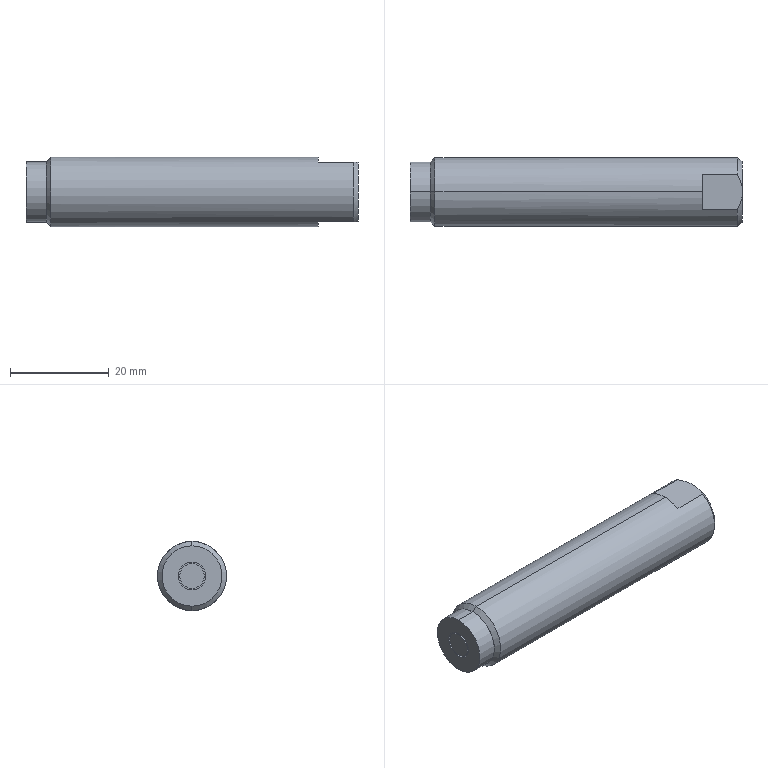Part | SolidWorks | features BaseBody 1 | 1 solid | 21 faces | box 67.1 x 14 x 14 mm | volume 10065 mm3 | plane 9 | cylinder 8 | cone 4 | commonest cylinder face diameters 5 x2 5.6 x2 12.2 x2 14 x2
STEP:
#1=CARTESIAN_POINT('',(59.1,3.606,-6.));
#2=VERTEX_POINT('',#1);
#3=CARTESIAN_POINT('',(59.1,0.,-7.));
#4=VERTEX_POINT('',#3);
#5=CARTESIAN_POINT('',(59.1,0.,0.));
#6=DIRECTION('',(-1.,0.,0.));
#7=DIRECTION('',(0.,0.,1.));
#8=AXIS2_PLACEMENT_3D('',#5,#6,#7);
#9=CIRCLE('',#8,7.);
#10=EDGE_CURVE('',#2,#4,#9,.T.);
#11=ORIENTED_EDGE('',*,*,#10,.T.);
#12=CARTESIAN_POINT('',(5.05,0.,-7.));
#13=VERTEX_POINT('',#12);
#14=CARTESIAN_POINT('',(67.1,0.,-7.));
#15=DIRECTION('',(-1.,0.,0.));
#16=VECTOR('',#15,1000.);
#17=LINE('',#14,#16);
#18=EDGE_CURVE('',#4,#13,#17,.T.);
#19=ORIENTED_EDGE('',*,*,#18,.T.);
#20=CARTESIAN_POINT('',(5.05,0.,7.));
#21=VERTEX_POINT('',#20);
#22=CARTESIAN_POINT('',(5.05,0.,0.));
#23=DIRECTION('',(1.,0.,0.));
#24=DIRECTION('',(0.,0.,1.));
#25=AXIS2_PLACEMENT_3D('',#22,#23,#24);
#26=CIRCLE('',#25,7.);
#27=EDGE_CURVE('',#13,#21,#26,.T.);
#28=ORIENTED_EDGE('',*,*,#27,.T.);
#29=CARTESIAN_POINT('',(59.1,0.,7.));
#30=VERTEX_POINT('',#29);
#31=CARTESIAN_POINT('',(67.1,0.,7.));
#32=DIRECTION('',(-1.,0.,0.));
#33=VECTOR('',#32,1000.);
#34=LINE('',#31,#33);
#35=EDGE_CURVE('',#30,#21,#34,.T.);
#36=ORIENTED_EDGE('',*,*,#35,.F.);
#37=CARTESIAN_POINT('',(59.1,3.606,6.));
#38=VERTEX_POINT('',#37);
#39=CARTESIAN_POINT('',(59.1,0.,0.));
#40=DIRECTION('',(-1.,0.,0.));
#41=DIRECTION('',(0.,0.,1.));
#42=AXIS2_PLACEMENT_3D('',#39,#40,#41);
#43=CIRCLE('',#42,7.);
#44=EDGE_CURVE('',#30,#38,#43,.T.);
#45=ORIENTED_EDGE('',*,*,#44,.T.);
#46=CARTESIAN_POINT('',(66.18,3.606,6.));
#47=VERTEX_POINT('',#46);
#48=CARTESIAN_POINT('',(67.1,3.606,6.));
#49=DIRECTION('',(1.,0.,0.));
#50=VECTOR('',#49,1000.);
#51=LINE('',#48,#50);
#52=EDGE_CURVE('',#38,#47,#51,.T.);
#53=ORIENTED_EDGE('',*,*,#52,.T.);
#54=CARTESIAN_POINT('',(66.18,3.606,-6.));
#55=VERTEX_POINT('',#54);
#56=CARTESIAN_POINT('',(66.18,0.,0.));
#57=DIRECTION('',(-1.,0.,0.));
#58=DIRECTION('',(0.,0.,1.));
#59=AXIS2_PLACEMENT_3D('',#56,#57,#58);
#60=CIRCLE('',#59,7.);
#61=EDGE_CURVE('',#47,#55,#60,.T.);
#62=ORIENTED_EDGE('',*,*,#61,.T.);
#63=CARTESIAN_POINT('',(67.1,3.606,-6.));
#64=DIRECTION('',(-1.,0.,0.));
#65=VECTOR('',#64,1000.);
#66=LINE('',#63,#65);
#67=EDGE_CURVE('',#55,#2,#66,.T.);
#68=ORIENTED_EDGE('',*,*,#67,.T.);
#69=EDGE_LOOP('',(#11,#19,#28,#36,#45,#53,#62,#68));
#70=FACE_OUTER_BOUND('',#69,.T.);
#71=CARTESIAN_POINT('',(67.1,0.,0.));
#72=DIRECTION('',(-1.,0.,0.));
#73=DIRECTION('',(0.,0.,1.));
#74=AXIS2_PLACEMENT_3D('',#71,#72,#73);
#75=CYLINDRICAL_SURFACE('',#74,7.);
#76=ADVANCED_FACE('',(#70),#75,.T.);
#77=CARTESIAN_POINT('',(4.13,0.,-6.08));
#78=VERTEX_POINT('',#77);
#79=CARTESIAN_POINT('',(4.13,0.,6.08));
#80=VERTEX_POINT('',#79);
#81=CARTESIAN_POINT('',(4.13,0.,0.));
#82=DIRECTION('',(1.,0.,0.));
#83=DIRECTION('',(0.,0.,-1.));
#84=AXIS2_PLACEMENT_3D('',#81,#82,#83);
#85=CIRCLE('',#84,6.08);
#86=EDGE_CURVE('',#78,#80,#85,.T.);
#87=ORIENTED_EDGE('',*,*,#86,.T.);
#88=CARTESIAN_POINT('',(5.05,0.,7.));
#89=DIRECTION('',(0.7071,0.,0.7071));
#90=VECTOR('',#89,1000.);
#91=LINE('',#88,#90);
#92=EDGE_CURVE('',#80,#21,#91,.T.);
#93=ORIENTED_EDGE('',*,*,#92,.T.);
#94=ORIENTED_EDGE('',*,*,#27,.F.);
#95=CARTESIAN_POINT('',(5.05,0.,-7.));
#96=DIRECTION('',(0.7071,0.,-0.7071));
#97=VECTOR('',#96,1000.);
#98=LINE('',#95,#97);
#99=EDGE_CURVE('',#78,#13,#98,.T.);
#100=ORIENTED_EDGE('',*,*,#99,.F.);
#101=EDGE_LOOP('',(#87,#93,#94,#100));
#102=FACE_OUTER_BOUND('',#101,.T.);
#103=CARTESIAN_POINT('',(5.05,0.,0.));
#104=DIRECTION('',(1.,0.,0.));
#105=DIRECTION('',(0.,0.,-1.));
#106=AXIS2_PLACEMENT_3D('',#103,#104,#105);
#107=CONICAL_SURFACE('',#106,7.,0.7854);
#108=ADVANCED_FACE('',(#102),#107,.T.);
#109=CARTESIAN_POINT('',(4.13,0.,6.1));
#110=VERTEX_POINT('',#109);
#111=CARTESIAN_POINT('',(4.13,0.,-6.1));
#112=VERTEX_POINT('',#111);
#113=CARTESIAN_POINT('',(4.13,0.,0.));
#114=DIRECTION('',(-1.,0.,0.));
#115=DIRECTION('',(0.,0.,1.));
#116=AXIS2_PLACEMENT_3D('',#113,#114,#115);
#117=CIRCLE('',#116,6.1);
#118=EDGE_CURVE('',#110,#112,#117,.T.);
#119=ORIENTED_EDGE('',*,*,#118,.T.);
#120=CARTESIAN_POINT('',(0.,0.,-6.1));
#121=VERTEX_POINT('',#120);
#122=CARTESIAN_POINT('',(67.1,0.,-6.1));
#123=DIRECTION('',(-1.,0.,0.));
#124=VECTOR('',#123,1000.);
#125=LINE('',#122,#124);
#126=EDGE_CURVE('',#112,#121,#125,.T.);
#127=ORIENTED_EDGE('',*,*,#126,.T.);
#128=CARTESIAN_POINT('',(0.,0.,6.1));
#129=VERTEX_POINT('',#128);
#130=CARTESIAN_POINT('',(0.,0.,0.));
#131=DIRECTION('',(1.,0.,0.));
#132=DIRECTION('',(0.,0.,1.));
#133=AXIS2_PLACEMENT_3D('',#130,#131,#132);
#134=CIRCLE('',#133,6.1);
#135=EDGE_CURVE('',#121,#129,#134,.T.);
#136=ORIENTED_EDGE('',*,*,#135,.T.);
#137=CARTESIAN_POINT('',(67.1,0.,6.1));
#138=DIRECTION('',(-1.,0.,0.));
#139=VECTOR('',#138,1000.);
#140=LINE('',#137,#139);
#141=EDGE_CURVE('',#110,#129,#140,.T.);
#142=ORIENTED_EDGE('',*,*,#141,.F.);
#143=EDGE_LOOP('',(#119,#127,#136,#142));
#144=FACE_OUTER_BOUND('',#143,.T.);
#145=CARTESIAN_POINT('',(67.1,0.,0.));
#146=DIRECTION('',(-1.,0.,0.));
#147=DIRECTION('',(0.,0.,1.));
#148=AXIS2_PLACEMENT_3D('',#145,#146,#147);
#149=CYLINDRICAL_SURFACE('',#148,6.1);
#150=ADVANCED_FACE('',(#144),#149,.T.);
#151=CARTESIAN_POINT('',(0.,0.,-2.8));
#152=VERTEX_POINT('',#151);
#153=CARTESIAN_POINT('',(0.,0.,2.8));
#154=VERTEX_POINT('',#153);
#155=CARTESIAN_POINT('',(0.,0.,0.));
#156=DIRECTION('',(-1.,0.,0.));
#157=DIRECTION('',(0.,0.,-1.));
#158=AXIS2_PLACEMENT_3D('',#155,#156,#157);
#159=CIRCLE('',#158,2.8);
#160=EDGE_CURVE('',#152,#154,#159,.T.);
#161=ORIENTED_EDGE('',*,*,#160,.T.);
#162=CARTESIAN_POINT('',(0.5,0.,2.8));
#163=VERTEX_POINT('',#162);
#164=CARTESIAN_POINT('',(0.5,0.,2.8));
#165=DIRECTION('',(1.,0.,0.));
#166=VECTOR('',#165,1000.);
#167=LINE('',#164,#166);
#168=EDGE_CURVE('',#154,#163,#167,.T.);
#169=ORIENTED_EDGE('',*,*,#168,.T.);
#170=CARTESIAN_POINT('',(0.5,0.,-2.8));
#171=VERTEX_POINT('',#170);
#172=CARTESIAN_POINT('',(0.5,0.,0.));
#173=DIRECTION('',(-1.,0.,0.));
#174=DIRECTION('',(0.,0.,-1.));
#175=AXIS2_PLACEMENT_3D('',#172,#173,#174);
#176=CIRCLE('',#175,2.8);
#177=EDGE_CURVE('',#171,#163,#176,.T.);
#178=ORIENTED_EDGE('',*,*,#177,.F.);
#179=CARTESIAN_POINT('',(0.5,0.,-2.8));
#180=DIRECTION('',(1.,0.,0.));
#181=VECTOR('',#180,1000.);
#182=LINE('',#179,#181);
#183=EDGE_CURVE('',#152,#171,#182,.T.);
#184=ORIENTED_EDGE('',*,*,#183,.F.);
#185=EDGE_LOOP('',(#161,#169,#178,#184));
#186=FACE_OUTER_BOUND('',#185,.T.);
#187=CARTESIAN_POINT('',(0.5,0.,0.));
#188=DIRECTION('',(1.,0.,0.));
#189=DIRECTION('',(0.,0.,-1.));
#190=AXIS2_PLACEMENT_3D('',#187,#188,#189);
#191=CYLINDRICAL_SURFACE('',#190,2.8);
#192=ADVANCED_FACE('',(#186),#191,.F.);
#193=CARTESIAN_POINT('',(0.,0.,-2.5));
#194=VERTEX_POINT('',#193);
#195=CARTESIAN_POINT('',(0.,0.,2.5));
#196=VERTEX_POINT('',#195);
#197=CARTESIAN_POINT('',(0.,0.,0.));
#198=DIRECTION('',(1.,0.,0.));
#199=DIRECTION('',(0.,0.,-1.));
#200=AXIS2_PLACEMENT_3D('',#197,#198,#199);
#201=CIRCLE('',#200,2.5);
#202=EDGE_CURVE('',#194,#196,#201,.T.);
#203=ORIENTED_EDGE('',*,*,#202,.T.);
#204=CARTESIAN_POINT('',(0.5,0.,2.5));
#205=VERTEX_POINT('',#204);
#206=CARTESIAN_POINT('',(0.5,0.,2.5));
#207=DIRECTION('',(1.,0.,0.));
#208=VECTOR('',#207,1000.);
#209=LINE('',#206,#208);
#210=EDGE_CURVE('',#196,#205,#209,.T.);
#211=ORIENTED_EDGE('',*,*,#210,.T.);
#212=CARTESIAN_POINT('',(0.5,0.,-2.5));
#213=VERTEX_POINT('',#212);
#214=CARTESIAN_POINT('',(0.5,0.,0.));
#215=DIRECTION('',(-1.,0.,0.));
#216=DIRECTION('',(0.,0.,-1.));
#217=AXIS2_PLACEMENT_3D('',#214,#215,#216);
#218=CIRCLE('',#217,2.5);
#219=EDGE_CURVE('',#205,#213,#218,.T.);
#220=ORIENTED_EDGE('',*,*,#219,.T.);
#221=CARTESIAN_POINT('',(0.5,0.,-2.5));
#222=DIRECTION('',(1.,0.,0.));
#223=VECTOR('',#222,1000.);
#224=LINE('',#221,#223);
#225=EDGE_CURVE('',#194,#213,#224,.T.);
#226=ORIENTED_EDGE('',*,*,#225,.F.);
#227=EDGE_LOOP('',(#203,#211,#220,#226));
#228=FACE_OUTER_BOUND('',#227,.T.);
#229=CARTESIAN_POINT('',(0.5,0.,0.));
#230=DIRECTION('',(1.,0.,0.));
#231=DIRECTION('',(0.,0.,-1.));
#232=AXIS2_PLACEMENT_3D('',#229,#230,#231);
#233=CYLINDRICAL_SURFACE('',#232,2.5);
#234=ADVANCED_FACE('',(#228),#233,.T.);
#235=ORIENTED_EDGE('',*,*,#18,.F.);
#236=CARTESIAN_POINT('',(59.1,-3.606,-6.));
#237=VERTEX_POINT('',#236);
#238=CARTESIAN_POINT('',(59.1,0.,0.));
#239=DIRECTION('',(-1.,0.,0.));
#240=DIRECTION('',(0.,0.,1.));
#241=AXIS2_PLACEMENT_3D('',#238,#239,#240);
#242=CIRCLE('',#241,7.);
#243=EDGE_CURVE('',#4,#237,#242,.T.);
#244=ORIENTED_EDGE('',*,*,#243,.T.);
#245=CARTESIAN_POINT('',(66.18,-3.606,-6.));
#246=VERTEX_POINT('',#245);
#247=CARTESIAN_POINT('',(67.1,-3.606,-6.));
#248=DIRECTION('',(1.,0.,0.));
#249=VECTOR('',#248,1000.);
#250=LINE('',#247,#249);
#251=EDGE_CURVE('',#237,#246,#250,.T.);
#252=ORIENTED_EDGE('',*,*,#251,.T.);
#253=CARTESIAN_POINT('',(66.18,-3.606,6.));
#254=VERTEX_POINT('',#253);
#255=CARTESIAN_POINT('',(66.18,0.,0.));
#256=DIRECTION('',(-1.,0.,0.));
#257=DIRECTION('',(0.,0.,1.));
#258=AXIS2_PLACEMENT_3D('',#255,#256,#257);
#259=CIRCLE('',#258,7.);
#260=EDGE_CURVE('',#246,#254,#259,.T.);
#261=ORIENTED_EDGE('',*,*,#260,.T.);
#262=CARTESIAN_POINT('',(59.1,-3.606,6.));
#263=VERTEX_POINT('',#262);
#264=CARTESIAN_POINT('',(67.1,-3.606,6.));
#265=DIRECTION('',(-1.,0.,0.));
#266=VECTOR('',#265,1000.);
#267=LINE('',#264,#266);
#268=EDGE_CURVE('',#254,#263,#267,.T.);
#269=ORIENTED_EDGE('',*,*,#268,.T.);
#270=CARTESIAN_POINT('',(59.1,0.,0.));
#271=DIRECTION('',(-1.,0.,0.));
#272=DIRECTION('',(0.,0.,1.));
#273=AXIS2_PLACEMENT_3D('',#270,#271,#272);
#274=CIRCLE('',#273,7.);
#275=EDGE_CURVE('',#263,#30,#274,.T.);
#276=ORIENTED_EDGE('',*,*,#275,.T.);
#277=ORIENTED_EDGE('',*,*,#35,.T.);
#278=CARTESIAN_POINT('',(5.05,0.,0.));
#279=DIRECTION('',(1.,0.,0.));
#280=DIRECTION('',(0.,0.,1.));
#281=AXIS2_PLACEMENT_3D('',#278,#279,#280);
#282=CIRCLE('',#281,7.);
#283=EDGE_CURVE('',#21,#13,#282,.T.);
#284=ORIENTED_EDGE('',*,*,#283,.T.);
#285=EDGE_LOOP('',(#235,#244,#252,#261,#269,#276,#277,#284));
#286=FACE_OUTER_BOUND('',#285,.T.);
#287=CARTESIAN_POINT('',(67.1,0.,0.));
#288=DIRECTION('',(-1.,0.,0.));
#289=DIRECTION('',(0.,0.,1.));
#290=AXIS2_PLACEMENT_3D('',#287,#288,#289);
#291=CYLINDRICAL_SURFACE('',#290,7.);
#292=ADVANCED_FACE('',(#286),#291,.T.);
#293=ORIENTED_EDGE('',*,*,#92,.F.);
#294=CARTESIAN_POINT('',(4.13,0.,0.));
#295=DIRECTION('',(1.,0.,0.));
#296=DIRECTION('',(0.,0.,-1.));
#297=AXIS2_PLACEMENT_3D('',#294,#295,#296);
#298=CIRCLE('',#297,6.08);
#299=EDGE_CURVE('',#80,#78,#298,.T.);
#300=ORIENTED_EDGE('',*,*,#299,.T.);
#301=ORIENTED_EDGE('',*,*,#99,.T.);
#302=ORIENTED_EDGE('',*,*,#283,.F.);
#303=EDGE_LOOP('',(#293,#300,#301,#302));
#304=FACE_OUTER_BOUND('',#303,.T.);
#305=CARTESIAN_POINT('',(5.05,0.,0.));
#306=DIRECTION('',(1.,0.,0.));
#307=DIRECTION('',(0.,0.,-1.));
#308=AXIS2_PLACEMENT_3D('',#305,#306,#307);
#309=CONICAL_SURFACE('',#308,7.,0.7854);
#310=ADVANCED_FACE('',(#304),#309,.T.);
#311=CARTESIAN_POINT('',(59.1,3.606,6.));
#312=DIRECTION('',(0.,-1.,0.));
#313=VECTOR('',#312,1000.);
#314=LINE('',#311,#313);
#315=EDGE_CURVE('',#38,#263,#314,.T.);
#316=ORIENTED_EDGE('',*,*,#315,.T.);
#317=ORIENTED_EDGE('',*,*,#268,.F.);
#318=CARTESIAN_POINT('',(67.1,-0.9831,6.));
#319=VERTEX_POINT('',#318);
#320=CARTESIAN_POINT('',(66.18,-3.606,6.));
#321=CARTESIAN_POINT('',(66.394,-3.19,6.));
#322=CARTESIAN_POINT('',(66.586,-2.766,6.));
#323=CARTESIAN_POINT('',(66.901,-1.895,6.));
#324=CARTESIAN_POINT('',(67.025,-1.448,6.));
#325=CARTESIAN_POINT('',(67.1,-0.9831,6.));
#326=B_SPLINE_CURVE_WITH_KNOTS('',3,(#320,#321,#322,#323,#324,#325),.UNSPECIFIED.,.F.,.F.,(4,2,4),(0.,0.00139,0.002779),.UNSPECIFIED.);
#327=EDGE_CURVE('',#254,#319,#326,.T.);
#328=ORIENTED_EDGE('',*,*,#327,.T.);
#329=CARTESIAN_POINT('',(67.1,0.9831,6.));
#330=VERTEX_POINT('',#329);
#331=CARTESIAN_POINT('',(67.1,3.606,6.));
#332=DIRECTION('',(0.,1.,0.));
#333=VECTOR('',#332,1000.);
#334=LINE('',#331,#333);
#335=EDGE_CURVE('',#319,#330,#334,.T.);
#336=ORIENTED_EDGE('',*,*,#335,.T.);
#337=CARTESIAN_POINT('',(67.1,0.9831,6.));
#338=CARTESIAN_POINT('',(67.025,1.448,6.));
#339=CARTESIAN_POINT('',(66.901,1.895,6.));
#340=CARTESIAN_POINT('',(66.586,2.766,6.));
#341=CARTESIAN_POINT('',(66.394,3.19,6.));
#342=CARTESIAN_POINT('',(66.18,3.606,6.));
#343=B_SPLINE_CURVE_WITH_KNOTS('',3,(#337,#338,#339,#340,#341,#342),.UNSPECIFIED.,.F.,.F.,(4,2,4),(0.,0.00139,0.002779),.UNSPECIFIED.);
#344=EDGE_CURVE('',#330,#47,#343,.T.);
#345=ORIENTED_EDGE('',*,*,#344,.T.);
#346=ORIENTED_EDGE('',*,*,#52,.F.);
#347=EDGE_LOOP('',(#316,#317,#328,#336,#345,#346));
#348=FACE_OUTER_BOUND('',#347,.T.);
#349=CARTESIAN_POINT('',(59.1,3.606,6.));
#350=DIRECTION('',(0.,0.,1.));
#351=DIRECTION('',(1.,0.,0.));
#352=AXIS2_PLACEMENT_3D('',#349,#350,#351);
#353=PLANE('',#352);
#354=ADVANCED_FACE('',(#348),#353,.T.);
#355=ORIENTED_EDGE('',*,*,#275,.F.);
#356=ORIENTED_EDGE('',*,*,#315,.F.);
#357=ORIENTED_EDGE('',*,*,#44,.F.);
#358=EDGE_LOOP('',(#355,#356,#357));
#359=FACE_OUTER_BOUND('',#358,.T.);
#360=CARTESIAN_POINT('',(59.1,0.,0.));
#361=DIRECTION('',(1.,0.,0.));
#362=DIRECTION('',(0.,0.,-1.));
#363=AXIS2_PLACEMENT_3D('',#360,#361,#362);
#364=PLANE('',#363);
#365=ADVANCED_FACE('',(#359),#364,.T.);
#366=ORIENTED_EDGE('',*,*,#327,.F.);
#367=ORIENTED_EDGE('',*,*,#260,.F.);
#368=CARTESIAN_POINT('',(67.1,-0.9831,-6.));
#369=VERTEX_POINT('',#368);
#370=CARTESIAN_POINT('',(66.18,-3.606,-6.));
#371=CARTESIAN_POINT('',(66.394,-3.19,-6.));
#372=CARTESIAN_POINT('',(66.586,-2.766,-6.));
#373=CARTESIAN_POINT('',(66.901,-1.895,-6.));
#374=CARTESIAN_POINT('',(67.025,-1.448,-6.));
#375=CARTESIAN_POINT('',(67.1,-0.9831,-6.));
#376=B_SPLINE_CURVE_WITH_KNOTS('',3,(#370,#371,#372,#373,#374,#375),.UNSPECIFIED.,.F.,.F.,(4,2,4),(0.,0.00139,0.002779),.UNSPECIFIED.);
#377=EDGE_CURVE('',#246,#369,#376,.T.);
#378=ORIENTED_EDGE('',*,*,#377,.T.);
#379=CARTESIAN_POINT('',(67.1,0.,0.));
#380=DIRECTION('',(-1.,0.,0.));
#381=DIRECTION('',(0.,0.,1.));
#382=AXIS2_PLACEMENT_3D('',#379,#380,#381);
#383=CIRCLE('',#382,6.08);
#384=EDGE_CURVE('',#369,#319,#383,.T.);
#385=ORIENTED_EDGE('',*,*,#384,.T.);
#386=EDGE_LOOP('',(#366,#367,#378,#385));
#387=FACE_OUTER_BOUND('',#386,.T.);
#388=CARTESIAN_POINT('',(66.18,0.,0.));
#389=DIRECTION('',(-1.,0.,0.));
#390=DIRECTION('',(0.,0.,1.));
#391=AXIS2_PLACEMENT_3D('',#388,#389,#390);
#392=CONICAL_SURFACE('',#391,7.,0.7854);
#393=ADVANCED_FACE('',(#387),#392,.T.);
#394=CARTESIAN_POINT('',(59.1,-3.606,-6.));
#395=DIRECTION('',(0.,1.,0.));
#396=VECTOR('',#395,1000.);
#397=LINE('',#394,#396);
#398=EDGE_CURVE('',#237,#2,#397,.T.);
#399=ORIENTED_EDGE('',*,*,#398,.T.);
#400=ORIENTED_EDGE('',*,*,#67,.F.);
#401=CARTESIAN_POINT('',(67.1,0.9831,-6.));
#402=VERTEX_POINT('',#401);
#403=CARTESIAN_POINT('',(66.18,3.606,-6.));
#404=CARTESIAN_POINT('',(66.394,3.19,-6.));
#405=CARTESIAN_POINT('',(66.586,2.766,-6.));
#406=CARTESIAN_POINT('',(66.901,1.895,-6.));
#407=CARTESIAN_POINT('',(67.025,1.448,-6.));
#408=CARTESIAN_POINT('',(67.1,0.9831,-6.));
#409=B_SPLINE_CURVE_WITH_KNOTS('',3,(#403,#404,#405,#406,#407,#408),.UNSPECIFIED.,.F.,.F.,(4,2,4),(0.,0.00139,0.002779),.UNSPECIFIED.);
#410=EDGE_CURVE('',#55,#402,#409,.T.);
#411=ORIENTED_EDGE('',*,*,#410,.T.);
#412=CARTESIAN_POINT('',(67.1,-3.606,-6.));
#413=DIRECTION('',(0.,-1.,0.));
#414=VECTOR('',#413,1000.);
#415=LINE('',#412,#414);
#416=EDGE_CURVE('',#402,#369,#415,.T.);
#417=ORIENTED_EDGE('',*,*,#416,.T.);
#418=ORIENTED_EDGE('',*,*,#377,.F.);
#419=ORIENTED_EDGE('',*,*,#251,.F.);
#420=EDGE_LOOP('',(#399,#400,#411,#417,#418,#419));
#421=FACE_OUTER_BOUND('',#420,.T.);
#422=CARTESIAN_POINT('',(59.1,-3.606,-6.));
#423=DIRECTION('',(0.,0.,-1.));
#424=DIRECTION('',(-1.,0.,0.));
#425=AXIS2_PLACEMENT_3D('',#422,#423,#424);
#426=PLANE('',#425);
#427=ADVANCED_FACE('',(#421),#426,.T.);
#428=ORIENTED_EDGE('',*,*,#10,.F.);
#429=ORIENTED_EDGE('',*,*,#398,.F.);
#430=ORIENTED_EDGE('',*,*,#243,.F.);
#431=EDGE_LOOP('',(#428,#429,#430));
#432=FACE_OUTER_BOUND('',#431,.T.);
#433=CARTESIAN_POINT('',(59.1,0.,0.));
#434=DIRECTION('',(1.,0.,0.));
#435=DIRECTION('',(0.,0.,-1.));
#436=AXIS2_PLACEMENT_3D('',#433,#434,#435);
#437=PLANE('',#436);
#438=ADVANCED_FACE('',(#432),#437,.T.);
#439=ORIENTED_EDGE('',*,*,#410,.F.);
#440=ORIENTED_EDGE('',*,*,#61,.F.);
#441=ORIENTED_EDGE('',*,*,#344,.F.);
#442=CARTESIAN_POINT('',(67.1,0.,0.));
#443=DIRECTION('',(-1.,0.,0.));
#444=DIRECTION('',(0.,0.,1.));
#445=AXIS2_PLACEMENT_3D('',#442,#443,#444);
#446=CIRCLE('',#445,6.08);
#447=EDGE_CURVE('',#330,#402,#446,.T.);
#448=ORIENTED_EDGE('',*,*,#447,.T.);
#449=EDGE_LOOP('',(#439,#440,#441,#448));
#450=FACE_OUTER_BOUND('',#449,.T.);
#451=CARTESIAN_POINT('',(66.18,0.,0.));
#452=DIRECTION('',(-1.,0.,0.));
#453=DIRECTION('',(0.,0.,1.));
#454=AXIS2_PLACEMENT_3D('',#451,#452,#453);
#455=CONICAL_SURFACE('',#454,7.,0.7854);
#456=ADVANCED_FACE('',(#450),#455,.T.);
#457=ORIENTED_EDGE('',*,*,#118,.F.);
#458=CARTESIAN_POINT('',(4.13,0.,0.));
#459=DIRECTION('',(-1.,0.,0.));
#460=DIRECTION('',(0.,0.,1.));
#461=AXIS2_PLACEMENT_3D('',#458,#459,#460);
#462=CIRCLE('',#461,6.1);
#463=EDGE_CURVE('',#112,#110,#462,.T.);
#464=ORIENTED_EDGE('',*,*,#463,.F.);
#465=EDGE_LOOP('',(#457,#464));
#466=FACE_OUTER_BOUND('',#465,.T.);
#467=ORIENTED_EDGE('',*,*,#86,.F.);
#468=ORIENTED_EDGE('',*,*,#299,.F.);
#469=EDGE_LOOP('',(#467,#468));
#470=FACE_BOUND('',#469,.T.);
#471=CARTESIAN_POINT('',(4.13,6.1,0.));
#472=DIRECTION('',(-1.,0.,0.));
#473=DIRECTION('',(0.,0.,1.));
#474=AXIS2_PLACEMENT_3D('',#471,#472,#473);
#475=PLANE('',#474);
#476=ADVANCED_FACE('',(#466,#470),#475,.F.);
#477=ORIENTED_EDGE('',*,*,#447,.F.);
#478=ORIENTED_EDGE('',*,*,#335,.F.);
#479=ORIENTED_EDGE('',*,*,#384,.F.);
#480=ORIENTED_EDGE('',*,*,#416,.F.);
#481=EDGE_LOOP('',(#477,#478,#479,#480));
#482=FACE_OUTER_BOUND('',#481,.T.);
#483=CARTESIAN_POINT('',(67.1,6.08,0.));
#484=DIRECTION('',(-1.,0.,0.));
#485=DIRECTION('',(0.,0.,1.));
#486=AXIS2_PLACEMENT_3D('',#483,#484,#485);
#487=PLANE('',#486);
#488=ADVANCED_FACE('',(#482),#487,.F.);
#489=ORIENTED_EDGE('',*,*,#126,.F.);
#490=ORIENTED_EDGE('',*,*,#463,.T.);
#491=ORIENTED_EDGE('',*,*,#141,.T.);
#492=CARTESIAN_POINT('',(0.,0.,0.));
#493=DIRECTION('',(1.,0.,0.));
#494=DIRECTION('',(0.,0.,1.));
#495=AXIS2_PLACEMENT_3D('',#492,#493,#494);
#496=CIRCLE('',#495,6.1);
#497=EDGE_CURVE('',#129,#121,#496,.T.);
#498=ORIENTED_EDGE('',*,*,#497,.T.);
#499=EDGE_LOOP('',(#489,#490,#491,#498));
#500=FACE_OUTER_BOUND('',#499,.T.);
#501=CARTESIAN_POINT('',(67.1,0.,0.));
#502=DIRECTION('',(-1.,0.,0.));
#503=DIRECTION('',(0.,0.,1.));
#504=AXIS2_PLACEMENT_3D('',#501,#502,#503);
#505=CYLINDRICAL_SURFACE('',#504,6.1);
#506=ADVANCED_FACE('',(#500),#505,.T.);
#507=ORIENTED_EDGE('',*,*,#160,.F.);
#508=CARTESIAN_POINT('',(0.,0.,0.));
#509=DIRECTION('',(-1.,0.,0.));
#510=DIRECTION('',(0.,0.,-1.));
#511=AXIS2_PLACEMENT_3D('',#508,#509,#510);
#512=CIRCLE('',#511,2.8);
#513=EDGE_CURVE('',#154,#152,#512,.T.);
#514=ORIENTED_EDGE('',*,*,#513,.F.);
#515=EDGE_LOOP('',(#507,#514));
#516=FACE_BOUND('',#515,.T.);
#517=ORIENTED_EDGE('',*,*,#497,.F.);
#518=ORIENTED_EDGE('',*,*,#135,.F.);
#519=EDGE_LOOP('',(#517,#518));
#520=FACE_OUTER_BOUND('',#519,.T.);
#521=CARTESIAN_POINT('',(0.,0.,0.));
#522=DIRECTION('',(1.,0.,0.));
#523=DIRECTION('',(0.,0.,-1.));
#524=AXIS2_PLACEMENT_3D('',#521,#522,#523);
#525=PLANE('',#524);
#526=ADVANCED_FACE('',(#516,#520),#525,.F.);
#527=ORIENTED_EDGE('',*,*,#168,.F.);
#528=ORIENTED_EDGE('',*,*,#513,.T.);
#529=ORIENTED_EDGE('',*,*,#183,.T.);
#530=CARTESIAN_POINT('',(0.5,0.,0.));
#531=DIRECTION('',(-1.,0.,0.));
#532=DIRECTION('',(0.,0.,-1.));
#533=AXIS2_PLACEMENT_3D('',#530,#531,#532);
#534=CIRCLE('',#533,2.8);
#535=EDGE_CURVE('',#163,#171,#534,.T.);
#536=ORIENTED_EDGE('',*,*,#535,.F.);
#537=EDGE_LOOP('',(#527,#528,#529,#536));
#538=FACE_OUTER_BOUND('',#537,.T.);
#539=CARTESIAN_POINT('',(0.5,0.,0.));
#540=DIRECTION('',(1.,0.,0.));
#541=DIRECTION('',(0.,0.,-1.));
#542=AXIS2_PLACEMENT_3D('',#539,#540,#541);
#543=CYLINDRICAL_SURFACE('',#542,2.8);
#544=ADVANCED_FACE('',(#538),#543,.F.);
#545=ORIENTED_EDGE('',*,*,#177,.T.);
#546=ORIENTED_EDGE('',*,*,#535,.T.);
#547=EDGE_LOOP('',(#545,#546));
#548=FACE_OUTER_BOUND('',#547,.T.);
#549=CARTESIAN_POINT('',(0.5,0.,0.));
#550=DIRECTION('',(-1.,0.,0.));
#551=DIRECTION('',(0.,0.,-1.));
#552=AXIS2_PLACEMENT_3D('',#549,#550,#551);
#553=CIRCLE('',#552,2.5);
#554=EDGE_CURVE('',#213,#205,#553,.T.);
#555=ORIENTED_EDGE('',*,*,#554,.F.);
#556=ORIENTED_EDGE('',*,*,#219,.F.);
#557=EDGE_LOOP('',(#555,#556));
#558=FACE_BOUND('',#557,.T.);
#559=CARTESIAN_POINT('',(0.5,0.,0.));
#560=DIRECTION('',(1.,0.,0.));
#561=DIRECTION('',(0.,0.,-1.));
#562=AXIS2_PLACEMENT_3D('',#559,#560,#561);
#563=PLANE('',#562);
#564=ADVANCED_FACE('',(#548,#558),#563,.F.);
#565=ORIENTED_EDGE('',*,*,#210,.F.);
#566=CARTESIAN_POINT('',(0.,0.,0.));
#567=DIRECTION('',(1.,0.,0.));
#568=DIRECTION('',(0.,0.,-1.));
#569=AXIS2_PLACEMENT_3D('',#566,#567,#568);
#570=CIRCLE('',#569,2.5);
#571=EDGE_CURVE('',#196,#194,#570,.T.);
#572=ORIENTED_EDGE('',*,*,#571,.T.);
#573=ORIENTED_EDGE('',*,*,#225,.T.);
#574=ORIENTED_EDGE('',*,*,#554,.T.);
#575=EDGE_LOOP('',(#565,#572,#573,#574));
#576=FACE_OUTER_BOUND('',#575,.T.);
#577=CARTESIAN_POINT('',(0.5,0.,0.));
#578=DIRECTION('',(1.,0.,0.));
#579=DIRECTION('',(0.,0.,-1.));
#580=AXIS2_PLACEMENT_3D('',#577,#578,#579);
#581=CYLINDRICAL_SURFACE('',#580,2.5);
#582=ADVANCED_FACE('',(#576),#581,.T.);
#583=ORIENTED_EDGE('',*,*,#202,.F.);
#584=ORIENTED_EDGE('',*,*,#571,.F.);
#585=EDGE_LOOP('',(#583,#584));
#586=FACE_OUTER_BOUND('',#585,.T.);
#587=CARTESIAN_POINT('',(0.,0.,0.));
#588=DIRECTION('',(1.,0.,0.));
#589=DIRECTION('',(0.,0.,-1.));
#590=AXIS2_PLACEMENT_3D('',#587,#588,#589);
#591=PLANE('',#590);
#592=ADVANCED_FACE('',(#586),#591,.F.);
#593=CLOSED_SHELL('',(#76,#108,#150,#192,#234,#292,#310,#354,#365,#393,#427,#438,#456,#476,#488,#506,#526,#544,#564,#582,#592));
#594=MANIFOLD_SOLID_BREP('',#593);
#595=CARTESIAN_POINT('',(0.,0.,0.));
#596=DIRECTION('',(0.,0.,1.));
#597=DIRECTION('',(1.,0.,0.));
#598=AXIS2_PLACEMENT_3D('',#595,#596,#597);
#599=(LENGTH_UNIT()NAMED_UNIT(*)SI_UNIT(.MILLI.,.METRE.));
#600=UNCERTAINTY_MEASURE_WITH_UNIT(LENGTH_MEASURE(0.00001),#599,'','');
#601=(NAMED_UNIT(*)PLANE_ANGLE_UNIT()SI_UNIT($,.RADIAN.));
#602=(NAMED_UNIT(*)SI_UNIT($,.STERADIAN.)SOLID_ANGLE_UNIT());
#603=(GEOMETRIC_REPRESENTATION_CONTEXT(3)GLOBAL_UNCERTAINTY_ASSIGNED_CONTEXT((#600))GLOBAL_UNIT_ASSIGNED_CONTEXT((#599,#601,#602))REPRESENTATION_CONTEXT('',''));
#604=ADVANCED_BREP_SHAPE_REPRESENTATION('',(#594,#598),#603);